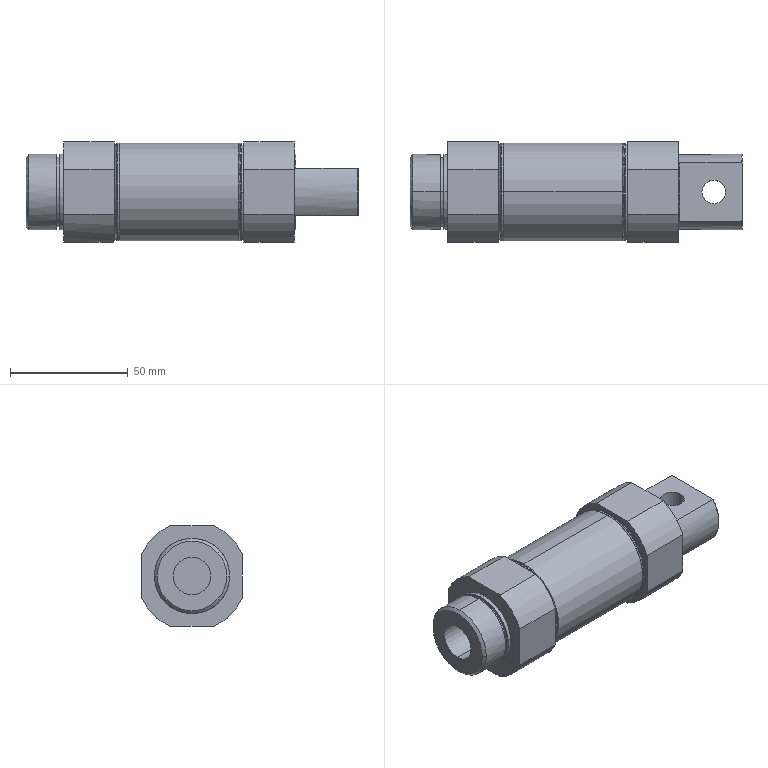Part | SolidWorks | features BaseBody 1 | 1 solid | 84 faces | box 141 x 42.5 x 42.5 mm | volume 117121 mm3 | cylinder 32 | plane 28 | cone 14 | spline 10 | commonest cylinder face diameters 46.5 x8 32 x6 41.6 x6 11.445 x4 10 x2 16 x2